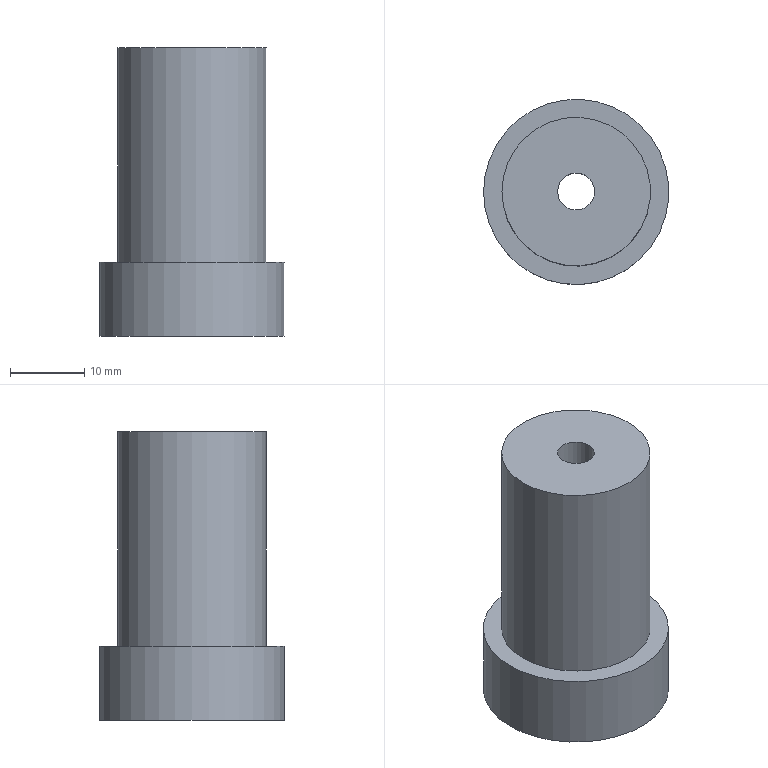Part | NX | features solid 2 | 1 solid | 8 faces | box 25 x 25 x 39 mm | volume 10158 mm3 | plane 4 | cylinder 4 | commonest cylinder face diameters 5 x1 15 x1 20.05 x1 25 x1
STEP:
#1=CARTESIAN_POINT('',(-1259.5,441.948,37.));
#2=VERTEX_POINT('',#1);
#3=CARTESIAN_POINT('',(-1262.,441.948,37.));
#4=DIRECTION('',(0.,0.,1.));
#5=DIRECTION('',(1.,0.,0.));
#6=AXIS2_PLACEMENT_3D('',#3,#4,#5);
#7=CIRCLE('',#6,2.5);
#8=EDGE_CURVE('',#2,#2,#7,.T.);
#9=ORIENTED_EDGE('',*,*,#8,.F.);
#10=EDGE_LOOP('',(#9));
#11=FACE_BOUND('',#10,.T.);
#12=CARTESIAN_POINT('',(-1272.025,441.948,37.));
#13=VERTEX_POINT('',#12);
#14=CARTESIAN_POINT('',(-1262.,441.948,37.));
#15=DIRECTION('',(0.,0.,-1.));
#16=DIRECTION('',(-1.,0.,0.));
#17=AXIS2_PLACEMENT_3D('',#14,#15,#16);
#18=CIRCLE('',#17,10.025);
#19=EDGE_CURVE('',#13,#13,#18,.F.);
#20=ORIENTED_EDGE('',*,*,#19,.T.);
#21=EDGE_LOOP('',(#20));
#22=FACE_BOUND('',#21,.T.);
#23=CARTESIAN_POINT('',(-1252.929,441.806,37.));
#24=DIRECTION('',(0.,0.,1.));
#25=DIRECTION('',(-1.,0.,0.));
#26=AXIS2_PLACEMENT_3D('',#23,#24,#25);
#27=PLANE('',#26);
#28=ADVANCED_FACE('',(#11,#22),#27,.T.);
#29=CARTESIAN_POINT('',(-1272.025,441.948,8.));
#30=VERTEX_POINT('',#29);
#31=CARTESIAN_POINT('',(-1262.,441.948,8.));
#32=DIRECTION('',(0.,0.,-1.));
#33=DIRECTION('',(-1.,0.,0.));
#34=AXIS2_PLACEMENT_3D('',#31,#32,#33);
#35=CIRCLE('',#34,10.025);
#36=EDGE_CURVE('',#30,#30,#35,.F.);
#37=ORIENTED_EDGE('',*,*,#36,.T.);
#38=EDGE_LOOP('',(#37));
#39=FACE_BOUND('',#38,.T.);
#40=ORIENTED_EDGE('',*,*,#19,.F.);
#41=EDGE_LOOP('',(#40));
#42=FACE_BOUND('',#41,.T.);
#43=CARTESIAN_POINT('',(-1262.,441.948,28.));
#44=DIRECTION('',(0.,0.,-1.));
#45=DIRECTION('',(1.,0.,0.));
#46=AXIS2_PLACEMENT_3D('',#43,#44,#45);
#47=CYLINDRICAL_SURFACE('',#46,10.025);
#48=ADVANCED_FACE('',(#39,#42),#47,.T.);
#49=CARTESIAN_POINT('',(-1274.5,441.948,-2.));
#50=VERTEX_POINT('',#49);
#51=CARTESIAN_POINT('',(-1262.,441.948,-2.));
#52=DIRECTION('',(0.,0.,-1.));
#53=DIRECTION('',(-1.,0.,0.));
#54=AXIS2_PLACEMENT_3D('',#51,#52,#53);
#55=CIRCLE('',#54,12.5);
#56=EDGE_CURVE('',#50,#50,#55,.F.);
#57=ORIENTED_EDGE('',*,*,#56,.F.);
#58=EDGE_LOOP('',(#57));
#59=FACE_BOUND('',#58,.T.);
#60=CARTESIAN_POINT('',(-1269.5,441.948,-2.));
#61=VERTEX_POINT('',#60);
#62=CARTESIAN_POINT('',(-1262.,441.948,-2.));
#63=DIRECTION('',(0.,0.,-1.));
#64=DIRECTION('',(-1.,0.,0.));
#65=AXIS2_PLACEMENT_3D('',#62,#63,#64);
#66=CIRCLE('',#65,7.5);
#67=EDGE_CURVE('',#61,#61,#66,.F.);
#68=ORIENTED_EDGE('',*,*,#67,.T.);
#69=EDGE_LOOP('',(#68));
#70=FACE_BOUND('',#69,.T.);
#71=CARTESIAN_POINT('',(-1262.,441.948,-2.));
#72=DIRECTION('',(0.,0.,1.));
#73=DIRECTION('',(-1.,0.,0.));
#74=AXIS2_PLACEMENT_3D('',#71,#72,#73);
#75=PLANE('',#74);
#76=ADVANCED_FACE('',(#59,#70),#75,.F.);
#77=ORIENTED_EDGE('',*,*,#36,.F.);
#78=EDGE_LOOP('',(#77));
#79=FACE_BOUND('',#78,.T.);
#80=CARTESIAN_POINT('',(-1274.5,441.948,8.));
#81=VERTEX_POINT('',#80);
#82=CARTESIAN_POINT('',(-1262.,441.948,8.));
#83=DIRECTION('',(0.,0.,-1.));
#84=DIRECTION('',(-1.,0.,0.));
#85=AXIS2_PLACEMENT_3D('',#82,#83,#84);
#86=CIRCLE('',#85,12.5);
#87=EDGE_CURVE('',#81,#81,#86,.F.);
#88=ORIENTED_EDGE('',*,*,#87,.T.);
#89=EDGE_LOOP('',(#88));
#90=FACE_BOUND('',#89,.T.);
#91=CARTESIAN_POINT('',(-1262.,441.948,8.));
#92=DIRECTION('',(0.,0.,1.));
#93=DIRECTION('',(-1.,0.,0.));
#94=AXIS2_PLACEMENT_3D('',#91,#92,#93);
#95=PLANE('',#94);
#96=ADVANCED_FACE('',(#79,#90),#95,.T.);
#97=ORIENTED_EDGE('',*,*,#56,.T.);
#98=EDGE_LOOP('',(#97));
#99=FACE_BOUND('',#98,.T.);
#100=ORIENTED_EDGE('',*,*,#87,.F.);
#101=EDGE_LOOP('',(#100));
#102=FACE_BOUND('',#101,.T.);
#103=CARTESIAN_POINT('',(-1262.,441.948,8.));
#104=DIRECTION('',(0.,0.,-1.));
#105=DIRECTION('',(1.,0.,0.));
#106=AXIS2_PLACEMENT_3D('',#103,#104,#105);
#107=CYLINDRICAL_SURFACE('',#106,12.5);
#108=ADVANCED_FACE('',(#99,#102),#107,.T.);
#109=CARTESIAN_POINT('',(-1259.5,441.948,18.));
#110=VERTEX_POINT('',#109);
#111=CARTESIAN_POINT('',(-1262.,441.948,18.));
#112=DIRECTION('',(0.,0.,1.));
#113=DIRECTION('',(1.,0.,0.));
#114=AXIS2_PLACEMENT_3D('',#111,#112,#113);
#115=CIRCLE('',#114,2.5);
#116=EDGE_CURVE('',#110,#110,#115,.T.);
#117=ORIENTED_EDGE('',*,*,#116,.T.);
#118=EDGE_LOOP('',(#117));
#119=FACE_BOUND('',#118,.T.);
#120=CARTESIAN_POINT('',(-1269.5,441.948,18.));
#121=VERTEX_POINT('',#120);
#122=CARTESIAN_POINT('',(-1262.,441.948,18.));
#123=DIRECTION('',(0.,0.,-1.));
#124=DIRECTION('',(-1.,0.,0.));
#125=AXIS2_PLACEMENT_3D('',#122,#123,#124);
#126=CIRCLE('',#125,7.5);
#127=EDGE_CURVE('',#121,#121,#126,.T.);
#128=ORIENTED_EDGE('',*,*,#127,.T.);
#129=EDGE_LOOP('',(#128));
#130=FACE_BOUND('',#129,.T.);
#131=CARTESIAN_POINT('',(-1262.,441.948,18.));
#132=DIRECTION('',(0.,0.,1.));
#133=DIRECTION('',(-1.,0.,0.));
#134=AXIS2_PLACEMENT_3D('',#131,#132,#133);
#135=PLANE('',#134);
#136=ADVANCED_FACE('',(#119,#130),#135,.F.);
#137=ORIENTED_EDGE('',*,*,#127,.F.);
#138=EDGE_LOOP('',(#137));
#139=FACE_BOUND('',#138,.T.);
#140=ORIENTED_EDGE('',*,*,#67,.F.);
#141=EDGE_LOOP('',(#140));
#142=FACE_BOUND('',#141,.T.);
#143=CARTESIAN_POINT('',(-1262.,441.948,8.));
#144=DIRECTION('',(0.,0.,1.));
#145=DIRECTION('',(-1.,0.,0.));
#146=AXIS2_PLACEMENT_3D('',#143,#144,#145);
#147=CYLINDRICAL_SURFACE('',#146,7.5);
#148=ADVANCED_FACE('',(#139,#142),#147,.F.);
#149=ORIENTED_EDGE('',*,*,#8,.T.);
#150=EDGE_LOOP('',(#149));
#151=FACE_BOUND('',#150,.T.);
#152=ORIENTED_EDGE('',*,*,#116,.F.);
#153=EDGE_LOOP('',(#152));
#154=FACE_BOUND('',#153,.T.);
#155=CARTESIAN_POINT('',(-1262.,441.948,-163.));
#156=DIRECTION('',(0.,0.,1.));
#157=DIRECTION('',(1.,0.,0.));
#158=AXIS2_PLACEMENT_3D('',#155,#156,#157);
#159=CYLINDRICAL_SURFACE('',#158,2.5);
#160=ADVANCED_FACE('',(#151,#154),#159,.F.);
#161=CLOSED_SHELL('',(#28,#48,#76,#96,#108,#136,#148,#160));
#162=MANIFOLD_SOLID_BREP('',#161);
#163=(LENGTH_UNIT()NAMED_UNIT(*)SI_UNIT(.MILLI.,.METRE.));
#164=UNCERTAINTY_MEASURE_WITH_UNIT(LENGTH_MEASURE(0.00001),#163,'','');
#165=(NAMED_UNIT(*)PLANE_ANGLE_UNIT()SI_UNIT($,.RADIAN.));
#166=(NAMED_UNIT(*)SI_UNIT($,.STERADIAN.)SOLID_ANGLE_UNIT());
#167=(GEOMETRIC_REPRESENTATION_CONTEXT(3)GLOBAL_UNCERTAINTY_ASSIGNED_CONTEXT((#164))GLOBAL_UNIT_ASSIGNED_CONTEXT((#163,#165,#166))REPRESENTATION_CONTEXT('',''));
#168=ADVANCED_BREP_SHAPE_REPRESENTATION('',(#162),#167);